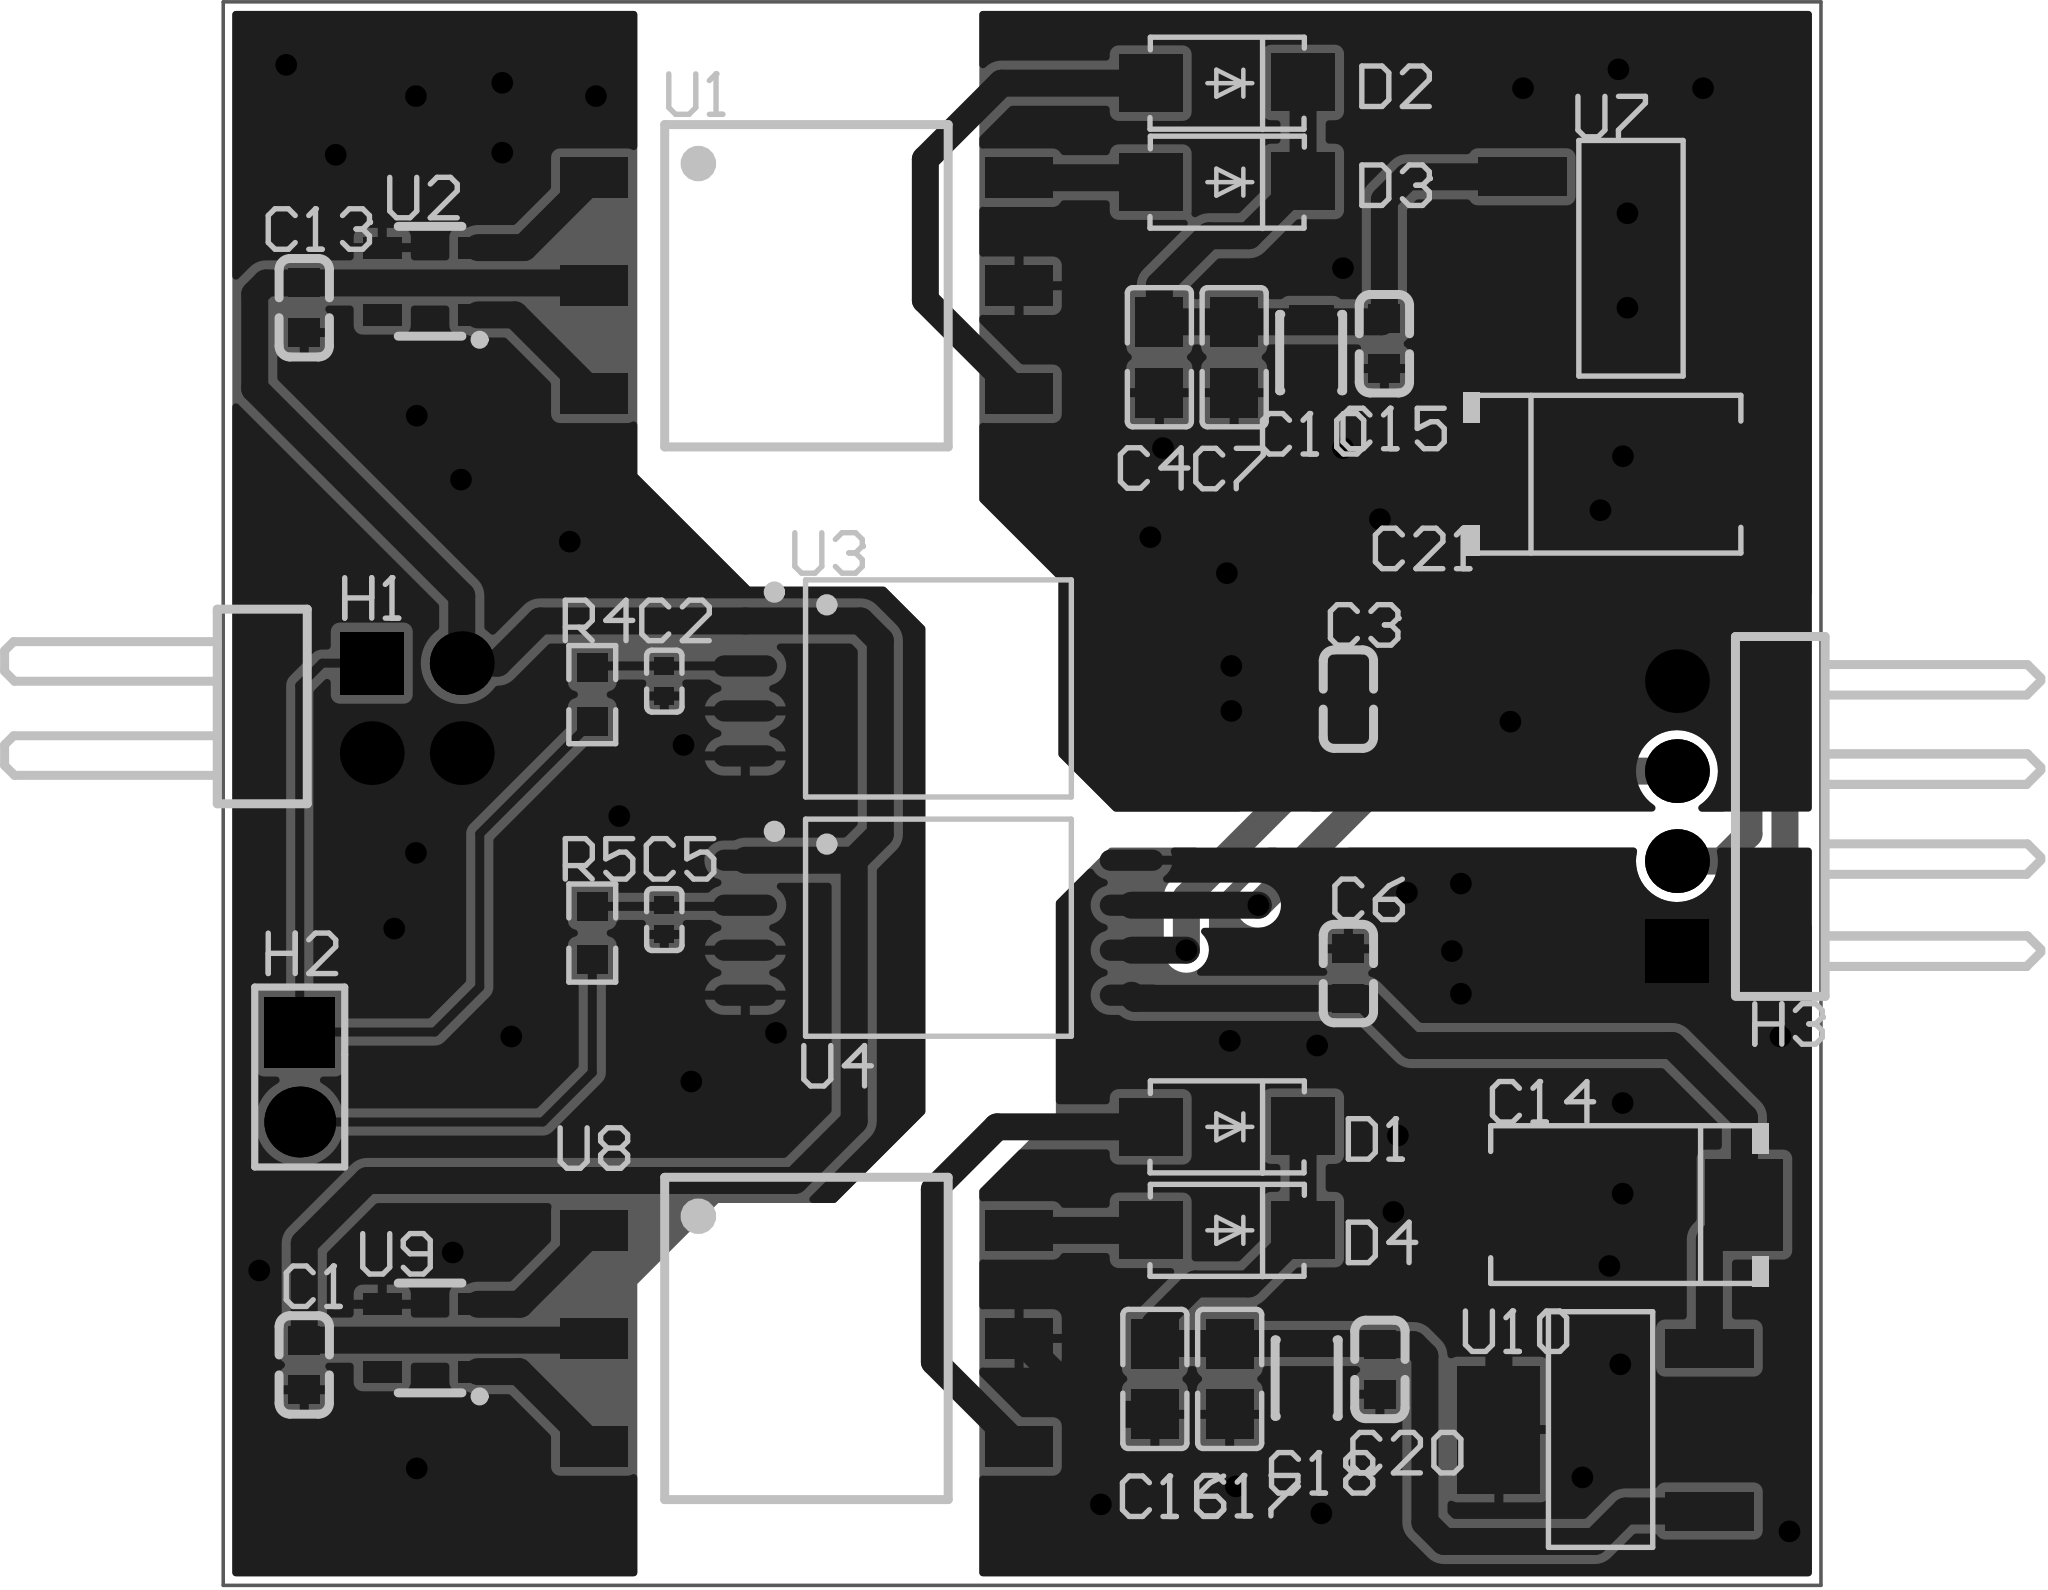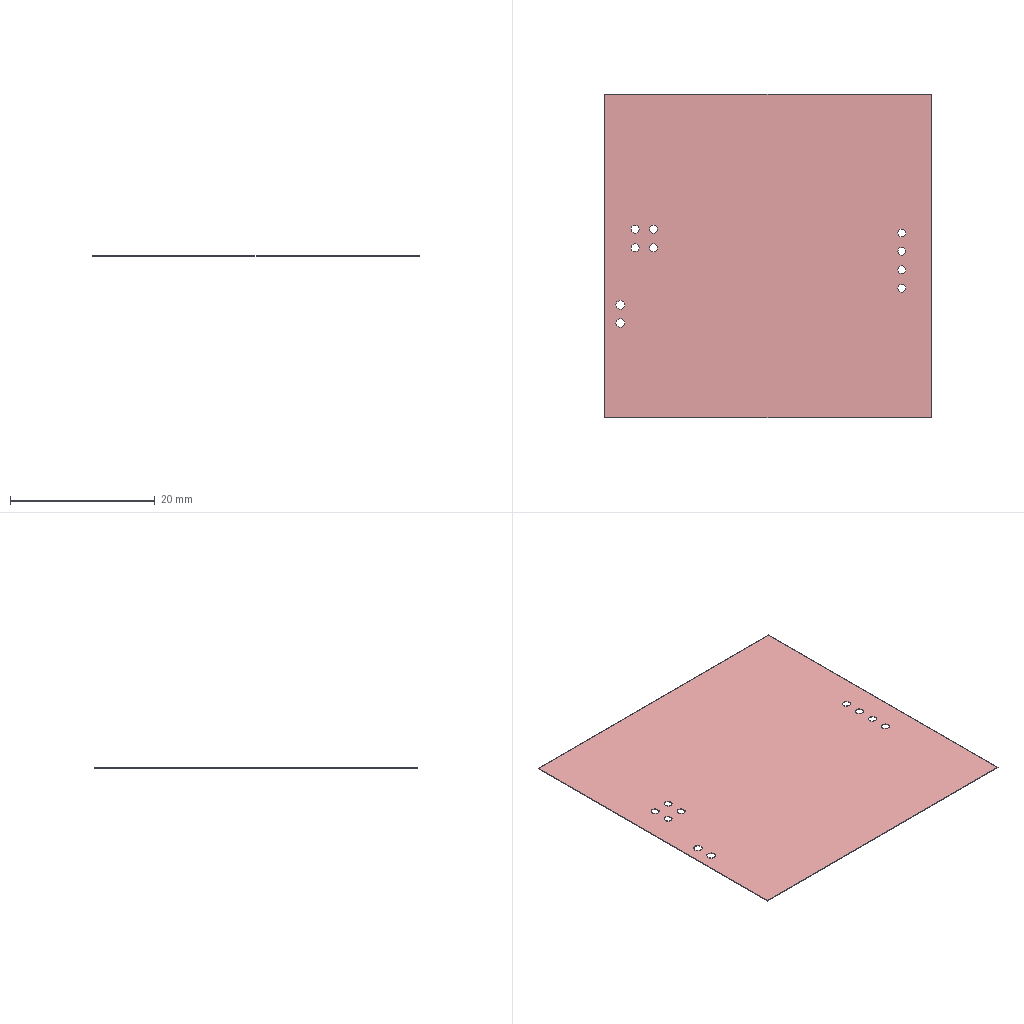Circuit board layout | Altium Designer | box 45.1 x 44.7 x 0.1 mm
Layer stack:
# Altium Designer layer stack of  (unit mm; dielectric type: 0 none, 1 core, 2 prepreg, 3 surface material)
index,name,kind,layer,copper_thickness_mm,dielectric_type,dielectric_thickness_mm,dielectric_material,dielectric_constant
0,Top Paste Mask Layer,other,,,,,,
1,Top Silkscreen Layer,other,,,,,,
2,Top Solder Mask Layer,dielectric,,,3,0.01,,3.3
3,Top Layer,copper,Top Layer,0.035,,,,
4,Bottom Layer,copper,Bottom Layer,0.035,,,,
5,Bottom Solder Mask Layer,dielectric,,,3,0.01,,3.3
6,Bottom Silkscreen Layer,other,,,,,,
7,Bottom Paste Mask Layer,other,,,,,,
# drill layer pairs: low layer,high layer
drill_pair,Top Layer,Bottom Layer
Part placement:
Designator,Comment,Layer,Footprint,Center-X(mm),Center-Y(mm),Rotation
C1,10uF,TopLayer,C0603,85.09,86.233,270
C2,22pF,TopLayer,C0402,95.25,105.537,90
C3,100nF,TopLayer,C0603,114.554,105.029,270
C4,4.7uF,TopLayer,C0805,109.22,114.681,90
C5,22pF,TopLayer,C0402,95.25,98.806,90
C6,100nF,TopLayer,C0603,114.554,97.282,270
C7,4.7uF,TopLayer,C0805,111.331,114.681,90
C10,100nF,TopLayer,CAP-SMD_L2.0-W1.25,113.504,114.808,90
C13,100nF,TopLayer,C0603,85.09,116.078,270
C14,47uF,TopLayer,CAP-SMD_L7.3-W4.3-FD,122.293,90.76,180
C15,470nF,TopLayer,C0603,115.57,115.062,90
C16,4.7uF,TopLayer,C0805,109.093,85.838,90
C17,4.7uF,TopLayer,C0805,111.204,85.838,90
C18,100nF,TopLayer,CAP-SMD_L2.0-W1.25,113.377,85.857,90
C20,470nF,TopLayer,C0603,115.443,86.106,90
C21,47uF,TopLayer,CAP-SMD_L7.3-W4.3-FD,121.906,111.379,0
D1,SS34,TopLayer,SMA_L4.3-W2.6-LS5.0-FD,111.125,92.964,0
D2,SS34,TopLayer,SMA_L4.3-W2.6-LS5.0-FD,111.125,122.428,0
D3,SS34,TopLayer,SMA_L4.3-W2.6-LS5.0-FD,111.125,119.634,0
D4,SS34,TopLayer,SMA_L4.3-W2.6-LS5.0-FD,111.125,90.043,0
H1,PZ254R-12-4P,TopLayer,HDR-TH_4P-P2.54-H-M-R2-C2-S2.54,88.265,104.775,270
H2,PZ254V-11-02P,TopLayer,HDR-TH_2P-P2.54-V-M,84.963,94.361,270
H3,PZ254R-11-04P,TopLayer,HDR-TH_4P-P2.54-H-M-W10.4,123.825,101.727,90
R4,51Ω,TopLayer,R0603,93.218,105.156,90
R5,51Ω,TopLayer,R0603,93.218,98.425,90
U1,750342879,TopLayer,XFMR-SMD_6P-L9.1-W8.0-P3.05-LS13.0-TL,99.261,116.699,0
U2,SN6505BDBVR,TopLayer,SOT-23-6_L2.9-W1.6-P0.95-LS2.8-BR,88.641,116.826,0
U3,UCC5350MCQDWVRQ1,TopLayer,SOIC-8_L7.5-W5.9-P1.27-LS11.5-BL,102.986,105.331,270
U4,UCC5350MCQDWVRQ1,TopLayer,SOIC-8_L7.5-W5.9-P1.27-LS11.5-BL,102.986,98.577,270
U7,LM2940IMP-15/NOPB,TopLayer,SOT-223-3_L6.5-W3.4-P2.30-LS7.0-BR,122.428,117.475,180
U8,750342879,TopLayer,XFMR-SMD_6P-L9.1-W8.0-P3.05-LS13.0-TL,99.261,86.981,0
U9,SN6505BDBVR,TopLayer,SOT-23-6_L2.9-W1.6-P0.95-LS2.8-BR,88.641,86.995,0
U10,LM2940IMP-15/NOPB,TopLayer,SOT-223-3_L6.5-W3.4-P2.30-LS7.0-BR,121.77,84.409,0
Pad and via stacks:
# Altium Designer via and pad stacks of  (unit mm). Each distinct definition once, with the count of objects using it.
# via: kind,start_layer,end_layer,hole_mm,diameter_mm,mode(0 simple;1 top-mid-bottom;2 full stack),diameter_per_layer,count,example_net
# pad: kind,layer,hole_mm,hole_type(0 round;1 square;2 slot),plating,top_size,top_shape(1 round;2 rect;3 octagon;9 rounded rect),mid_size,bottom_size,mode,footprint,size_per_layer,count,example
pad,Top Layer,0,0,plated,0.8x0.9,2,0.8x0.9,0.8x0.9,0,C0603,,12,C1.2
pad,Top Layer,0,0,plated,0.5x0.54,2,0.5x0.54,0.5x0.54,0,C0402,,4,C2.2
pad,Top Layer,0,0,plated,1.41x1.35,2,1.41x1.35,1.41x1.35,0,C0805,,8,C4.2
pad,Top Layer,0,0,plated,1.25x0.7,2,1.25x0.7,1.25x0.7,0,CAP-SMD_L2.0-W1.25,,4,C10.1
pad,Top Layer,0,0,plated,2.185x2.592,2,2.185x2.592,2.185x2.592,0,CAP-SMD_L7.3-W4.3-FD,,4,C14.2
pad,Top Layer,0,0,plated,1.8x1.62,2,1.8x1.62,1.8x1.62,0,SMA_L4.3-W2.6-LS5.0-FD,,8,D1.1
pad,Top Layer,0,0,plated,0.8065x0.864,2,0.8065x0.864,0.8065x0.864,0,R0603,,4,R4.2
pad,Top Layer,0,0,plated,1.9x1.14,2,1.9x1.14,1.9x1.14,0,XFMR-SMD_6P-L9.1-W8.0-P3.05-LS13.0-TL,,12,U1.6
pad,Top Layer,0,0,plated,1.1x0.6,2,1.1x0.6,1.1x0.6,0,SOT-23-6_L2.9-W1.6-P0.95-LS2.8-BR,,12,U2.3
pad,Top Layer,0,0,plated,0.6x1.8,1,0.6x1.8,0.6x1.8,0,SOIC-8_L7.5-W5.9-P1.27-LS11.5-BL,,16,U3.1
pad,Top Layer,0,0,plated,2.5x1.1,2,2.5x1.1,2.5x1.1,0,SOT-223-3_L6.5-W3.4-P2.30-LS7.0-BR,,6,U7.1
pad,Top Layer,0,0,plated,2.34x3.6,2,2.34x3.6,2.34x3.6,0,SOT-223-3_L6.5-W3.4-P2.30-LS7.0-BR,,2,U7.4
pad,Multi-Layer,1.1,0,plated,1.778x1.8,2,1.778x1.8,1.778x1.8,0,HDR-TH_4P-P2.54-H-M-R2-C2-S2.54,,1,H1.1
pad,Multi-Layer,1.1,0,plated,1.8x1.8,1,1.8x1.8,1.8x1.8,0,HDR-TH_4P-P2.54-H-M-R2-C2-S2.54,,3,H1.2
pad,Multi-Layer,1.2,0,plated,2x2,2,2x2,2x2,0,HDR-TH_2P-P2.54-V-M,,1,H2.1
pad,Multi-Layer,1.2,0,plated,2x2,1,2x2,2x2,0,HDR-TH_2P-P2.54-V-M,,1,H2.2
pad,Multi-Layer,1.1,0,plated,1.8x1.8,2,1.8x1.8,1.8x1.8,0,HDR-TH_4P-P2.54-H-M-W10.4,,1,H3.1
pad,Multi-Layer,1.1,0,plated,1.8x1.8,1,1.8x1.8,1.8x1.8,0,HDR-TH_4P-P2.54-H-M-W10.4,,3,H3.2
via,Top Layer,Bottom Layer,0.3048,0.61,0,,55,CLAMP1_L
Copper pours:
name,layer,net,type(0 solid;1 hatched;2 none)
Top Layer-SGND,Top Layer,SGND,0
Top Layer-S1H_0V,Top Layer,S1H_0V,0
Top Layer-S1L_0V,Top Layer,S1L_0V,0
Bottom Layer-SGND,Bottom Layer,SGND,0
Bottom Layer-S1H_0V,Bottom Layer,S1H_0V,0
Bottom Layer-S1L_0V,Bottom Layer,S1L_0V,0
Design rules, without the lines most boards share:
# Altium Designer design rules of  (exported by Altium Designer, unit mm)
# columns: name | kind | enabled | priority | scope1 | scope2 | descriptor | typed fields (field=value)
Plane_innerPlane | 0 | disabled | 1 | All | All | Clearance Constraint (Gap=6mil) (Disabled)(All),(All) | gap=0.1524
Plane_innerPlane_1 | 63 | disabled | 1 | All | All | Board Clearance Constraint (Gap=0mil) (Disabled)(All) |
Copper_copperRegion | 0 | disabled | 2 | All | All | Clearance Constraint (Gap=6mil) (Disabled)(All),(All) | gap=0.1524
Copper_copperRegion_1 | 63 | disabled | 2 | All | All | Board Clearance Constraint (Gap=0mil) (Disabled)(All) |
copperThickness1oz | 0 | enabled | 3 | All | All | Clearance Constraint (Gap=6mil) (All),(All) | gap=0.1524
copperThickness1oz_1 | 63 | enabled | 3 | All | All | Board Clearance Constraint (Gap=0mil) (All) |
otherClearance | 52 | enabled | 1 | All | All | Hole To Hole Clearance (Gap=11.8mil) (All),(All) | gap=0.2997
copperThickness1oz_2 | 2 | enabled | 1 | All | All | Width Constraint (Min=5mil) (Max=100mil) (Preferred=10mil) (All) |
differentialPair | 51 | enabled | 1 | All | All | Differential Pairs Uncoupled Length using the Gap Constraints (Min=5mil) (Max=6mil) (Prefered=6mil)  and Width Constraints (Min=5mil) (Max=100mil) (Prefered=100mil) (All) |
copperRegion | 20 | enabled | 1 | (InNet('SGND') OR InNet('$1N9') OR InNet('$1N10')) | All | Polygon Connect Rule(Relief Connect )(Conductor Width=10mil) (Relief Angle=90 Angle) (Entries=4) (Air Gap Width=10mil) ((InNet('SGND') OR InNet('$1N9') OR InNet('$1N10'))),(All) | connect_style(0=relief,1=direct,2=none)=0 relief_conductor_width=0.254 relief_entries=4